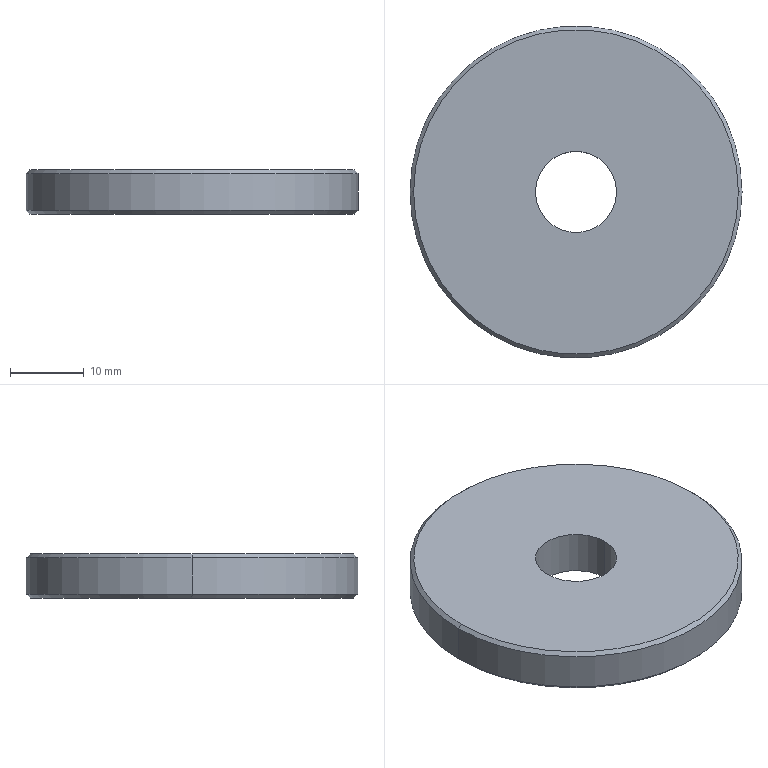Part | SolidWorks | features Chamfer 1, Extrusion 1 | 1 solid | 10 faces | box 45 x 45 x 6 mm | volume 8937 mm3 | cone 4 | cylinder 4 | plane 2 | commonest cylinder face diameters 11 x2 45 x2
STEP:
#1=CARTESIAN_POINT('',(22.,0.,6.));
#2=VERTEX_POINT('',#1);
#3=CARTESIAN_POINT('',(-22.,0.,6.));
#4=VERTEX_POINT('',#3);
#5=CARTESIAN_POINT('',(0.,0.,6.));
#6=DIRECTION('',(0.,0.,1.));
#7=DIRECTION('',(1.,0.,0.));
#8=AXIS2_PLACEMENT_3D('',#5,#6,#7);
#9=CIRCLE('',#8,22.);
#10=EDGE_CURVE('',#2,#4,#9,.T.);
#11=ORIENTED_EDGE('',*,*,#10,.F.);
#12=CARTESIAN_POINT('',(22.5,0.,5.5));
#13=VERTEX_POINT('',#12);
#14=CARTESIAN_POINT('',(22.,0.,6.));
#15=DIRECTION('',(0.7071,0.,-0.7071));
#16=VECTOR('',#15,1000.);
#17=LINE('',#14,#16);
#18=EDGE_CURVE('',#2,#13,#17,.T.);
#19=ORIENTED_EDGE('',*,*,#18,.T.);
#20=CARTESIAN_POINT('',(-22.5,0.,5.5));
#21=VERTEX_POINT('',#20);
#22=CARTESIAN_POINT('',(0.,0.,5.5));
#23=DIRECTION('',(0.,0.,-1.));
#24=DIRECTION('',(1.,0.,0.));
#25=AXIS2_PLACEMENT_3D('',#22,#23,#24);
#26=CIRCLE('',#25,22.5);
#27=EDGE_CURVE('',#21,#13,#26,.T.);
#28=ORIENTED_EDGE('',*,*,#27,.F.);
#29=CARTESIAN_POINT('',(-22.,0.,6.));
#30=DIRECTION('',(-0.7071,0.,-0.7071));
#31=VECTOR('',#30,1000.);
#32=LINE('',#29,#31);
#33=EDGE_CURVE('',#4,#21,#32,.T.);
#34=ORIENTED_EDGE('',*,*,#33,.F.);
#35=EDGE_LOOP('',(#11,#19,#28,#34));
#36=FACE_OUTER_BOUND('',#35,.T.);
#37=CARTESIAN_POINT('',(0.,0.,6.));
#38=DIRECTION('',(0.,0.,-1.));
#39=DIRECTION('',(-1.,0.,0.));
#40=AXIS2_PLACEMENT_3D('',#37,#38,#39);
#41=CONICAL_SURFACE('',#40,22.,0.7854);
#42=ADVANCED_FACE('',(#36),#41,.T.);
#43=CARTESIAN_POINT('',(-22.,0.,0.));
#44=VERTEX_POINT('',#43);
#45=CARTESIAN_POINT('',(22.,0.,0.));
#46=VERTEX_POINT('',#45);
#47=CARTESIAN_POINT('',(0.,0.,0.));
#48=DIRECTION('',(0.,0.,-1.));
#49=DIRECTION('',(1.,0.,0.));
#50=AXIS2_PLACEMENT_3D('',#47,#48,#49);
#51=CIRCLE('',#50,22.);
#52=EDGE_CURVE('',#44,#46,#51,.T.);
#53=ORIENTED_EDGE('',*,*,#52,.F.);
#54=CARTESIAN_POINT('',(-22.5,0.,0.5));
#55=VERTEX_POINT('',#54);
#56=CARTESIAN_POINT('',(-22.5,0.,0.5));
#57=DIRECTION('',(-0.7071,0.,0.7071));
#58=VECTOR('',#57,1000.);
#59=LINE('',#56,#58);
#60=EDGE_CURVE('',#44,#55,#59,.T.);
#61=ORIENTED_EDGE('',*,*,#60,.T.);
#62=CARTESIAN_POINT('',(22.5,0.,0.5));
#63=VERTEX_POINT('',#62);
#64=CARTESIAN_POINT('',(0.,0.,0.5));
#65=DIRECTION('',(0.,0.,1.));
#66=DIRECTION('',(1.,0.,0.));
#67=AXIS2_PLACEMENT_3D('',#64,#65,#66);
#68=CIRCLE('',#67,22.5);
#69=EDGE_CURVE('',#63,#55,#68,.T.);
#70=ORIENTED_EDGE('',*,*,#69,.F.);
#71=CARTESIAN_POINT('',(22.5,0.,0.5));
#72=DIRECTION('',(0.7071,0.,0.7071));
#73=VECTOR('',#72,1000.);
#74=LINE('',#71,#73);
#75=EDGE_CURVE('',#46,#63,#74,.T.);
#76=ORIENTED_EDGE('',*,*,#75,.F.);
#77=EDGE_LOOP('',(#53,#61,#70,#76));
#78=FACE_OUTER_BOUND('',#77,.T.);
#79=CARTESIAN_POINT('',(0.,0.,0.5));
#80=DIRECTION('',(0.,0.,1.));
#81=DIRECTION('',(1.,0.,0.));
#82=AXIS2_PLACEMENT_3D('',#79,#80,#81);
#83=CONICAL_SURFACE('',#82,22.5,0.7854);
#84=ADVANCED_FACE('',(#78),#83,.T.);
#85=CARTESIAN_POINT('',(-5.5,0.,6.));
#86=VERTEX_POINT('',#85);
#87=CARTESIAN_POINT('',(5.5,0.,6.));
#88=VERTEX_POINT('',#87);
#89=CARTESIAN_POINT('',(0.,0.,6.));
#90=DIRECTION('',(0.,0.,1.));
#91=DIRECTION('',(1.,0.,0.));
#92=AXIS2_PLACEMENT_3D('',#89,#90,#91);
#93=CIRCLE('',#92,5.5);
#94=EDGE_CURVE('',#86,#88,#93,.T.);
#95=ORIENTED_EDGE('',*,*,#94,.T.);
#96=CARTESIAN_POINT('',(5.5,0.,0.));
#97=VERTEX_POINT('',#96);
#98=CARTESIAN_POINT('',(5.5,0.,6.));
#99=DIRECTION('',(0.,0.,-1.));
#100=VECTOR('',#99,1000.);
#101=LINE('',#98,#100);
#102=EDGE_CURVE('',#88,#97,#101,.T.);
#103=ORIENTED_EDGE('',*,*,#102,.T.);
#104=CARTESIAN_POINT('',(-5.5,0.,0.));
#105=VERTEX_POINT('',#104);
#106=CARTESIAN_POINT('',(0.,0.,0.));
#107=DIRECTION('',(0.,0.,1.));
#108=DIRECTION('',(1.,0.,0.));
#109=AXIS2_PLACEMENT_3D('',#106,#107,#108);
#110=CIRCLE('',#109,5.5);
#111=EDGE_CURVE('',#105,#97,#110,.T.);
#112=ORIENTED_EDGE('',*,*,#111,.F.);
#113=CARTESIAN_POINT('',(-5.5,0.,6.));
#114=DIRECTION('',(0.,0.,-1.));
#115=VECTOR('',#114,1000.);
#116=LINE('',#113,#115);
#117=EDGE_CURVE('',#86,#105,#116,.T.);
#118=ORIENTED_EDGE('',*,*,#117,.F.);
#119=EDGE_LOOP('',(#95,#103,#112,#118));
#120=FACE_OUTER_BOUND('',#119,.T.);
#121=CARTESIAN_POINT('',(0.,0.,6.));
#122=DIRECTION('',(0.,0.,-1.));
#123=DIRECTION('',(-1.,0.,0.));
#124=AXIS2_PLACEMENT_3D('',#121,#122,#123);
#125=CYLINDRICAL_SURFACE('',#124,5.5);
#126=ADVANCED_FACE('',(#120),#125,.F.);
#127=ORIENTED_EDGE('',*,*,#27,.T.);
#128=CARTESIAN_POINT('',(22.5,0.,6.));
#129=DIRECTION('',(0.,0.,-1.));
#130=VECTOR('',#129,1000.);
#131=LINE('',#128,#130);
#132=EDGE_CURVE('',#13,#63,#131,.T.);
#133=ORIENTED_EDGE('',*,*,#132,.T.);
#134=ORIENTED_EDGE('',*,*,#69,.T.);
#135=CARTESIAN_POINT('',(-22.5,0.,6.));
#136=DIRECTION('',(0.,0.,-1.));
#137=VECTOR('',#136,1000.);
#138=LINE('',#135,#137);
#139=EDGE_CURVE('',#21,#55,#138,.T.);
#140=ORIENTED_EDGE('',*,*,#139,.F.);
#141=EDGE_LOOP('',(#127,#133,#134,#140));
#142=FACE_OUTER_BOUND('',#141,.T.);
#143=CARTESIAN_POINT('',(0.,0.,6.));
#144=DIRECTION('',(0.,0.,-1.));
#145=DIRECTION('',(-1.,0.,0.));
#146=AXIS2_PLACEMENT_3D('',#143,#144,#145);
#147=CYLINDRICAL_SURFACE('',#146,22.5);
#148=ADVANCED_FACE('',(#142),#147,.T.);
#149=CARTESIAN_POINT('',(0.,0.,6.));
#150=DIRECTION('',(0.,0.,1.));
#151=DIRECTION('',(1.,0.,0.));
#152=AXIS2_PLACEMENT_3D('',#149,#150,#151);
#153=CIRCLE('',#152,22.);
#154=EDGE_CURVE('',#4,#2,#153,.T.);
#155=ORIENTED_EDGE('',*,*,#154,.T.);
#156=ORIENTED_EDGE('',*,*,#10,.T.);
#157=EDGE_LOOP('',(#155,#156));
#158=FACE_OUTER_BOUND('',#157,.T.);
#159=ORIENTED_EDGE('',*,*,#94,.F.);
#160=CARTESIAN_POINT('',(0.,0.,6.));
#161=DIRECTION('',(0.,0.,1.));
#162=DIRECTION('',(1.,0.,0.));
#163=AXIS2_PLACEMENT_3D('',#160,#161,#162);
#164=CIRCLE('',#163,5.5);
#165=EDGE_CURVE('',#88,#86,#164,.T.);
#166=ORIENTED_EDGE('',*,*,#165,.F.);
#167=EDGE_LOOP('',(#159,#166));
#168=FACE_BOUND('',#167,.T.);
#169=CARTESIAN_POINT('',(0.,0.,6.));
#170=DIRECTION('',(0.,0.,1.));
#171=DIRECTION('',(1.,0.,0.));
#172=AXIS2_PLACEMENT_3D('',#169,#170,#171);
#173=PLANE('',#172);
#174=ADVANCED_FACE('',(#158,#168),#173,.T.);
#175=CARTESIAN_POINT('',(0.,0.,0.));
#176=DIRECTION('',(0.,0.,-1.));
#177=DIRECTION('',(1.,0.,0.));
#178=AXIS2_PLACEMENT_3D('',#175,#176,#177);
#179=CIRCLE('',#178,22.);
#180=EDGE_CURVE('',#46,#44,#179,.T.);
#181=ORIENTED_EDGE('',*,*,#180,.T.);
#182=ORIENTED_EDGE('',*,*,#52,.T.);
#183=EDGE_LOOP('',(#181,#182));
#184=FACE_OUTER_BOUND('',#183,.T.);
#185=ORIENTED_EDGE('',*,*,#111,.T.);
#186=CARTESIAN_POINT('',(0.,0.,0.));
#187=DIRECTION('',(0.,0.,1.));
#188=DIRECTION('',(1.,0.,0.));
#189=AXIS2_PLACEMENT_3D('',#186,#187,#188);
#190=CIRCLE('',#189,5.5);
#191=EDGE_CURVE('',#97,#105,#190,.T.);
#192=ORIENTED_EDGE('',*,*,#191,.T.);
#193=EDGE_LOOP('',(#185,#192));
#194=FACE_BOUND('',#193,.T.);
#195=CARTESIAN_POINT('',(0.,0.,0.));
#196=DIRECTION('',(0.,0.,1.));
#197=DIRECTION('',(1.,0.,0.));
#198=AXIS2_PLACEMENT_3D('',#195,#196,#197);
#199=PLANE('',#198);
#200=ADVANCED_FACE('',(#184,#194),#199,.F.);
#201=ORIENTED_EDGE('',*,*,#132,.F.);
#202=CARTESIAN_POINT('',(0.,0.,5.5));
#203=DIRECTION('',(0.,0.,-1.));
#204=DIRECTION('',(1.,0.,0.));
#205=AXIS2_PLACEMENT_3D('',#202,#203,#204);
#206=CIRCLE('',#205,22.5);
#207=EDGE_CURVE('',#13,#21,#206,.T.);
#208=ORIENTED_EDGE('',*,*,#207,.T.);
#209=ORIENTED_EDGE('',*,*,#139,.T.);
#210=CARTESIAN_POINT('',(0.,0.,0.5));
#211=DIRECTION('',(0.,0.,1.));
#212=DIRECTION('',(1.,0.,0.));
#213=AXIS2_PLACEMENT_3D('',#210,#211,#212);
#214=CIRCLE('',#213,22.5);
#215=EDGE_CURVE('',#55,#63,#214,.T.);
#216=ORIENTED_EDGE('',*,*,#215,.T.);
#217=EDGE_LOOP('',(#201,#208,#209,#216));
#218=FACE_OUTER_BOUND('',#217,.T.);
#219=CARTESIAN_POINT('',(0.,0.,6.));
#220=DIRECTION('',(0.,0.,-1.));
#221=DIRECTION('',(-1.,0.,0.));
#222=AXIS2_PLACEMENT_3D('',#219,#220,#221);
#223=CYLINDRICAL_SURFACE('',#222,22.5);
#224=ADVANCED_FACE('',(#218),#223,.T.);
#225=ORIENTED_EDGE('',*,*,#102,.F.);
#226=ORIENTED_EDGE('',*,*,#165,.T.);
#227=ORIENTED_EDGE('',*,*,#117,.T.);
#228=ORIENTED_EDGE('',*,*,#191,.F.);
#229=EDGE_LOOP('',(#225,#226,#227,#228));
#230=FACE_OUTER_BOUND('',#229,.T.);
#231=CARTESIAN_POINT('',(0.,0.,6.));
#232=DIRECTION('',(0.,0.,-1.));
#233=DIRECTION('',(-1.,0.,0.));
#234=AXIS2_PLACEMENT_3D('',#231,#232,#233);
#235=CYLINDRICAL_SURFACE('',#234,5.5);
#236=ADVANCED_FACE('',(#230),#235,.F.);
#237=ORIENTED_EDGE('',*,*,#60,.F.);
#238=ORIENTED_EDGE('',*,*,#180,.F.);
#239=ORIENTED_EDGE('',*,*,#75,.T.);
#240=ORIENTED_EDGE('',*,*,#215,.F.);
#241=EDGE_LOOP('',(#237,#238,#239,#240));
#242=FACE_OUTER_BOUND('',#241,.T.);
#243=CARTESIAN_POINT('',(0.,0.,0.5));
#244=DIRECTION('',(0.,0.,1.));
#245=DIRECTION('',(1.,0.,0.));
#246=AXIS2_PLACEMENT_3D('',#243,#244,#245);
#247=CONICAL_SURFACE('',#246,22.5,0.7854);
#248=ADVANCED_FACE('',(#242),#247,.T.);
#249=ORIENTED_EDGE('',*,*,#18,.F.);
#250=ORIENTED_EDGE('',*,*,#154,.F.);
#251=ORIENTED_EDGE('',*,*,#33,.T.);
#252=ORIENTED_EDGE('',*,*,#207,.F.);
#253=EDGE_LOOP('',(#249,#250,#251,#252));
#254=FACE_OUTER_BOUND('',#253,.T.);
#255=CARTESIAN_POINT('',(0.,0.,6.));
#256=DIRECTION('',(0.,0.,-1.));
#257=DIRECTION('',(-1.,0.,0.));
#258=AXIS2_PLACEMENT_3D('',#255,#256,#257);
#259=CONICAL_SURFACE('',#258,22.,0.7854);
#260=ADVANCED_FACE('',(#254),#259,.T.);
#261=CLOSED_SHELL('',(#42,#84,#126,#148,#174,#200,#224,#236,#248,#260));
#262=MANIFOLD_SOLID_BREP('',#261);
#263=CARTESIAN_POINT('',(0.,0.,0.));
#264=DIRECTION('',(0.,0.,1.));
#265=DIRECTION('',(1.,0.,0.));
#266=AXIS2_PLACEMENT_3D('',#263,#264,#265);
#267=(LENGTH_UNIT()NAMED_UNIT(*)SI_UNIT(.MILLI.,.METRE.));
#268=UNCERTAINTY_MEASURE_WITH_UNIT(LENGTH_MEASURE(0.00001),#267,'','');
#269=(NAMED_UNIT(*)PLANE_ANGLE_UNIT()SI_UNIT($,.RADIAN.));
#270=(NAMED_UNIT(*)SI_UNIT($,.STERADIAN.)SOLID_ANGLE_UNIT());
#271=(GEOMETRIC_REPRESENTATION_CONTEXT(3)GLOBAL_UNCERTAINTY_ASSIGNED_CONTEXT((#268))GLOBAL_UNIT_ASSIGNED_CONTEXT((#267,#269,#270))REPRESENTATION_CONTEXT('',''));
#272=ADVANCED_BREP_SHAPE_REPRESENTATION('',(#262,#266),#271);